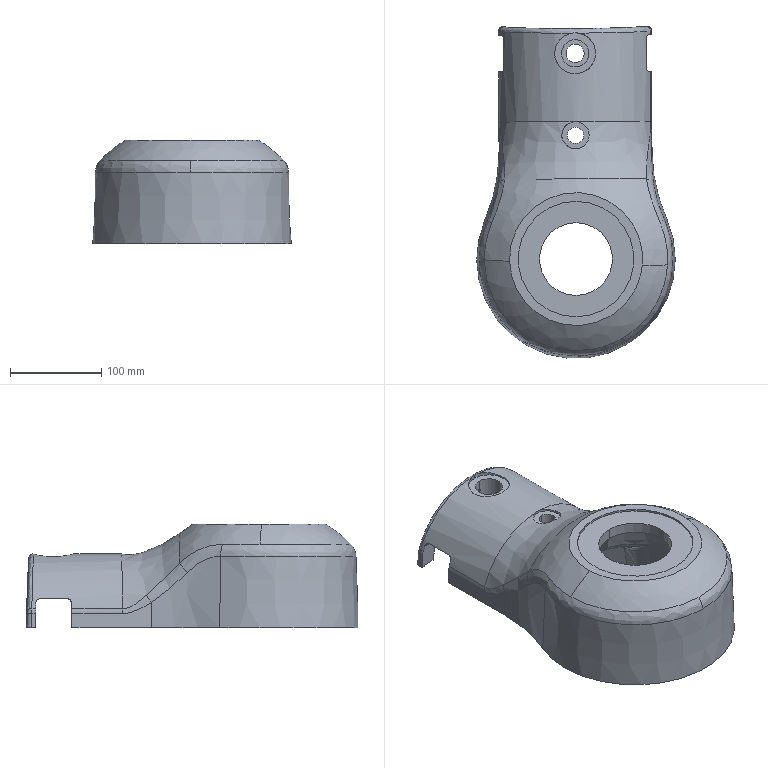Part | SolidWorks | features BaseBody 1 | 1 solid | 157 faces | box 217.971 x 365.089 x 114.123 mm | volume 2199337 mm3 | cone 51 | cylinder 43 | plane 39 | spline 24 | commonest cylinder face diameters 10 x13 20 x6 30 x4 40 x4 4 x2 18 x2